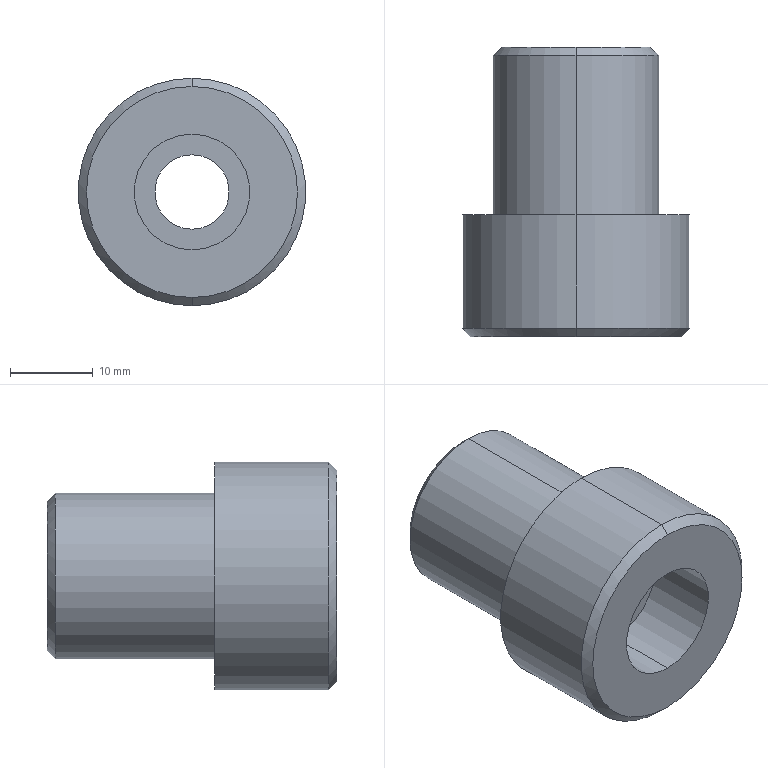Part | Creo | 1 solid | 16 faces | box 27.5 x 35 x 27.5 mm | volume 12011 mm3 | cylinder 8 | plane 4 | cone 4 | commonest cylinder face diameters 9 x2 14 x2 20 x2 27.5 x2
STEP:
#1=CARTESIAN_POINT('',(0.,0.,0.));
#2=DIRECTION('',(0.,0.,1.));
#3=DIRECTION('',(1.,0.,0.));
#4=AXIS2_PLACEMENT_3D('',#1,#2,#3);
#5=CARTESIAN_POINT('',(-64.528,-214.,-110.));
#6=VERTEX_POINT('',#5);
#7=CARTESIAN_POINT('',(-64.528,-214.,-92.));
#8=VERTEX_POINT('',#7);
#9=CARTESIAN_POINT('',(-64.528,-214.,-101.));
#10=DIRECTION('',(0.,1.,0.));
#11=DIRECTION('',(0.,0.,-1.));
#12=AXIS2_PLACEMENT_3D('',#9,#10,#11);
#13=CIRCLE('',#12,9.);
#14=EDGE_CURVE('',#6,#8,#13,.T.);
#15=ORIENTED_EDGE('',*,*,#14,.F.);
#16=CARTESIAN_POINT('',(-64.528,-214.,-101.));
#17=DIRECTION('',(0.,1.,0.));
#18=DIRECTION('',(0.,0.,1.));
#19=AXIS2_PLACEMENT_3D('',#16,#17,#18);
#20=CIRCLE('',#19,9.);
#21=EDGE_CURVE('',#8,#6,#20,.T.);
#22=ORIENTED_EDGE('',*,*,#21,.F.);
#23=EDGE_LOOP('',(#15,#22));
#24=FACE_OUTER_BOUND('',#23,.F.);
#25=CARTESIAN_POINT('',(-64.528,-214.,-96.5));
#26=VERTEX_POINT('',#25);
#27=CARTESIAN_POINT('',(-64.528,-214.,-105.5));
#28=VERTEX_POINT('',#27);
#29=CARTESIAN_POINT('',(-64.528,-214.,-101.));
#30=DIRECTION('',(0.,-1.,0.));
#31=DIRECTION('',(0.,0.,1.));
#32=AXIS2_PLACEMENT_3D('',#29,#30,#31);
#33=CIRCLE('',#32,4.5);
#34=EDGE_CURVE('',#26,#28,#33,.T.);
#35=ORIENTED_EDGE('',*,*,#34,.F.);
#36=CARTESIAN_POINT('',(-64.528,-214.,-101.));
#37=DIRECTION('',(0.,-1.,0.));
#38=DIRECTION('',(0.,0.,-1.));
#39=AXIS2_PLACEMENT_3D('',#36,#37,#38);
#40=CIRCLE('',#39,4.5);
#41=EDGE_CURVE('',#28,#26,#40,.T.);
#42=ORIENTED_EDGE('',*,*,#41,.F.);
#43=EDGE_LOOP('',(#35,#42));
#44=FACE_BOUND('',#43,.F.);
#45=CARTESIAN_POINT('',(-64.528,-214.,-101.));
#46=DIRECTION('',(0.,-1.,0.));
#47=DIRECTION('',(0.,0.,1.));
#48=AXIS2_PLACEMENT_3D('',#45,#46,#47);
#49=PLANE('',#48);
#50=ADVANCED_FACE('',(#24,#44),#49,.F.);
#51=CARTESIAN_POINT('',(-64.528,-215.,-111.));
#52=VERTEX_POINT('',#51);
#53=CARTESIAN_POINT('',(-64.528,-215.,-91.));
#54=VERTEX_POINT('',#53);
#55=CARTESIAN_POINT('',(-64.528,-215.,-101.));
#56=DIRECTION('',(0.,1.,0.));
#57=DIRECTION('',(0.,0.,-1.));
#58=AXIS2_PLACEMENT_3D('',#55,#56,#57);
#59=CIRCLE('',#58,10.);
#60=EDGE_CURVE('',#52,#54,#59,.T.);
#61=ORIENTED_EDGE('',*,*,#60,.F.);
#62=CARTESIAN_POINT('',(-64.528,-214.,-110.));
#63=DIRECTION('',(0.,-0.7071,-0.7071));
#64=VECTOR('',#63,1.414);
#65=LINE('',#62,#64);
#66=EDGE_CURVE('',#6,#52,#65,.T.);
#67=ORIENTED_EDGE('',*,*,#66,.F.);
#68=ORIENTED_EDGE('',*,*,#14,.T.);
#69=CARTESIAN_POINT('',(-64.528,-214.,-92.));
#70=DIRECTION('',(0.,-0.7071,0.7071));
#71=VECTOR('',#70,1.414);
#72=LINE('',#69,#71);
#73=EDGE_CURVE('',#8,#54,#72,.T.);
#74=ORIENTED_EDGE('',*,*,#73,.T.);
#75=EDGE_LOOP('',(#61,#67,#68,#74));
#76=FACE_OUTER_BOUND('',#75,.F.);
#77=CARTESIAN_POINT('',(-64.528,-214.5,-101.));
#78=DIRECTION('',(0.,-1.,0.));
#79=DIRECTION('',(0.,0.,-1.));
#80=AXIS2_PLACEMENT_3D('',#77,#78,#79);
#81=CONICAL_SURFACE('',#80,9.5,45.);
#82=ADVANCED_FACE('',(#76),#81,.T.);
#83=ORIENTED_EDGE('',*,*,#60,.T.);
#84=CARTESIAN_POINT('',(-64.528,-234.25,-91.));
#85=VERTEX_POINT('',#84);
#86=CARTESIAN_POINT('',(-64.528,-234.25,-91.));
#87=DIRECTION('',(0.,1.,0.));
#88=VECTOR('',#87,19.25);
#89=LINE('',#86,#88);
#90=EDGE_CURVE('',#85,#54,#89,.T.);
#91=ORIENTED_EDGE('',*,*,#90,.F.);
#92=CARTESIAN_POINT('',(-64.528,-234.25,-111.));
#93=VERTEX_POINT('',#92);
#94=CARTESIAN_POINT('',(-64.528,-234.25,-101.));
#95=DIRECTION('',(0.,-1.,0.));
#96=DIRECTION('',(0.,0.,1.));
#97=AXIS2_PLACEMENT_3D('',#94,#95,#96);
#98=CIRCLE('',#97,10.);
#99=EDGE_CURVE('',#85,#93,#98,.T.);
#100=ORIENTED_EDGE('',*,*,#99,.T.);
#101=CARTESIAN_POINT('',(-64.528,-234.25,-111.));
#102=DIRECTION('',(0.,1.,0.));
#103=VECTOR('',#102,19.25);
#104=LINE('',#101,#103);
#105=EDGE_CURVE('',#93,#52,#104,.T.);
#106=ORIENTED_EDGE('',*,*,#105,.T.);
#107=EDGE_LOOP('',(#83,#91,#100,#106));
#108=FACE_OUTER_BOUND('',#107,.F.);
#109=CARTESIAN_POINT('',(-64.528,-249.,-101.));
#110=DIRECTION('',(0.,1.,0.));
#111=DIRECTION('',(0.,0.,-1.));
#112=AXIS2_PLACEMENT_3D('',#109,#110,#111);
#113=CYLINDRICAL_SURFACE('',#112,10.);
#114=ADVANCED_FACE('',(#108),#113,.T.);
#115=CARTESIAN_POINT('',(-64.528,-215.,-101.));
#116=DIRECTION('',(0.,1.,0.));
#117=DIRECTION('',(0.,0.,1.));
#118=AXIS2_PLACEMENT_3D('',#115,#116,#117);
#119=CIRCLE('',#118,10.);
#120=EDGE_CURVE('',#54,#52,#119,.T.);
#121=ORIENTED_EDGE('',*,*,#120,.T.);
#122=ORIENTED_EDGE('',*,*,#105,.F.);
#123=CARTESIAN_POINT('',(-64.528,-234.25,-101.));
#124=DIRECTION('',(0.,-1.,0.));
#125=DIRECTION('',(0.,0.,-1.));
#126=AXIS2_PLACEMENT_3D('',#123,#124,#125);
#127=CIRCLE('',#126,10.);
#128=EDGE_CURVE('',#93,#85,#127,.T.);
#129=ORIENTED_EDGE('',*,*,#128,.T.);
#130=ORIENTED_EDGE('',*,*,#90,.T.);
#131=EDGE_LOOP('',(#121,#122,#129,#130));
#132=FACE_OUTER_BOUND('',#131,.F.);
#133=CARTESIAN_POINT('',(-64.528,-249.,-101.));
#134=DIRECTION('',(0.,1.,0.));
#135=DIRECTION('',(0.,0.,-1.));
#136=AXIS2_PLACEMENT_3D('',#133,#134,#135);
#137=CYLINDRICAL_SURFACE('',#136,10.);
#138=ADVANCED_FACE('',(#132),#137,.T.);
#139=ORIENTED_EDGE('',*,*,#120,.F.);
#140=ORIENTED_EDGE('',*,*,#73,.F.);
#141=ORIENTED_EDGE('',*,*,#21,.T.);
#142=ORIENTED_EDGE('',*,*,#66,.T.);
#143=EDGE_LOOP('',(#139,#140,#141,#142));
#144=FACE_OUTER_BOUND('',#143,.F.);
#145=CARTESIAN_POINT('',(-64.528,-214.5,-101.));
#146=DIRECTION('',(0.,-1.,0.));
#147=DIRECTION('',(0.,0.,-1.));
#148=AXIS2_PLACEMENT_3D('',#145,#146,#147);
#149=CONICAL_SURFACE('',#148,9.5,45.);
#150=ADVANCED_FACE('',(#144),#149,.T.);
#151=CARTESIAN_POINT('',(-64.528,-234.25,-114.75));
#152=VERTEX_POINT('',#151);
#153=CARTESIAN_POINT('',(-64.528,-234.25,-87.25));
#154=VERTEX_POINT('',#153);
#155=CARTESIAN_POINT('',(-64.528,-234.25,-101.));
#156=DIRECTION('',(0.,1.,0.));
#157=DIRECTION('',(0.,0.,-1.));
#158=AXIS2_PLACEMENT_3D('',#155,#156,#157);
#159=CIRCLE('',#158,13.75);
#160=EDGE_CURVE('',#152,#154,#159,.T.);
#161=ORIENTED_EDGE('',*,*,#160,.F.);
#162=CARTESIAN_POINT('',(-64.528,-234.25,-101.));
#163=DIRECTION('',(0.,1.,0.));
#164=DIRECTION('',(0.,0.,1.));
#165=AXIS2_PLACEMENT_3D('',#162,#163,#164);
#166=CIRCLE('',#165,13.75);
#167=EDGE_CURVE('',#154,#152,#166,.T.);
#168=ORIENTED_EDGE('',*,*,#167,.F.);
#169=EDGE_LOOP('',(#161,#168));
#170=FACE_OUTER_BOUND('',#169,.F.);
#171=ORIENTED_EDGE('',*,*,#99,.F.);
#172=ORIENTED_EDGE('',*,*,#128,.F.);
#173=EDGE_LOOP('',(#171,#172));
#174=FACE_BOUND('',#173,.F.);
#175=CARTESIAN_POINT('',(-64.528,-234.25,-101.));
#176=DIRECTION('',(0.,-1.,0.));
#177=DIRECTION('',(0.,0.,1.));
#178=AXIS2_PLACEMENT_3D('',#175,#176,#177);
#179=PLANE('',#178);
#180=ADVANCED_FACE('',(#170,#174),#179,.F.);
#181=CARTESIAN_POINT('',(-64.528,-248.,-87.25));
#182=VERTEX_POINT('',#181);
#183=CARTESIAN_POINT('',(-64.528,-248.,-114.75));
#184=VERTEX_POINT('',#183);
#185=CARTESIAN_POINT('',(-64.528,-248.,-101.));
#186=DIRECTION('',(0.,-1.,0.));
#187=DIRECTION('',(0.,0.,1.));
#188=AXIS2_PLACEMENT_3D('',#185,#186,#187);
#189=CIRCLE('',#188,13.75);
#190=EDGE_CURVE('',#182,#184,#189,.T.);
#191=ORIENTED_EDGE('',*,*,#190,.T.);
#192=CARTESIAN_POINT('',(-64.528,-248.,-114.75));
#193=DIRECTION('',(0.,1.,0.));
#194=VECTOR('',#193,13.75);
#195=LINE('',#192,#194);
#196=EDGE_CURVE('',#184,#152,#195,.T.);
#197=ORIENTED_EDGE('',*,*,#196,.T.);
#198=ORIENTED_EDGE('',*,*,#160,.T.);
#199=CARTESIAN_POINT('',(-64.528,-248.,-87.25));
#200=DIRECTION('',(0.,1.,0.));
#201=VECTOR('',#200,13.75);
#202=LINE('',#199,#201);
#203=EDGE_CURVE('',#182,#154,#202,.T.);
#204=ORIENTED_EDGE('',*,*,#203,.F.);
#205=EDGE_LOOP('',(#191,#197,#198,#204));
#206=FACE_OUTER_BOUND('',#205,.F.);
#207=CARTESIAN_POINT('',(-64.528,-249.,-101.));
#208=DIRECTION('',(0.,1.,0.));
#209=DIRECTION('',(0.,0.,-1.));
#210=AXIS2_PLACEMENT_3D('',#207,#208,#209);
#211=CYLINDRICAL_SURFACE('',#210,13.75);
#212=ADVANCED_FACE('',(#206),#211,.T.);
#213=ORIENTED_EDGE('',*,*,#190,.F.);
#214=CARTESIAN_POINT('',(-64.528,-249.,-88.25));
#215=VERTEX_POINT('',#214);
#216=CARTESIAN_POINT('',(-64.528,-249.,-88.25));
#217=DIRECTION('',(0.,0.7071,0.7071));
#218=VECTOR('',#217,1.414);
#219=LINE('',#216,#218);
#220=EDGE_CURVE('',#215,#182,#219,.T.);
#221=ORIENTED_EDGE('',*,*,#220,.F.);
#222=CARTESIAN_POINT('',(-64.528,-249.,-113.75));
#223=VERTEX_POINT('',#222);
#224=CARTESIAN_POINT('',(-64.528,-249.,-101.));
#225=DIRECTION('',(0.,-1.,0.));
#226=DIRECTION('',(0.,0.,1.));
#227=AXIS2_PLACEMENT_3D('',#224,#225,#226);
#228=CIRCLE('',#227,12.75);
#229=EDGE_CURVE('',#215,#223,#228,.T.);
#230=ORIENTED_EDGE('',*,*,#229,.T.);
#231=CARTESIAN_POINT('',(-64.528,-249.,-113.75));
#232=DIRECTION('',(0.,0.7071,-0.7071));
#233=VECTOR('',#232,1.414);
#234=LINE('',#231,#233);
#235=EDGE_CURVE('',#223,#184,#234,.T.);
#236=ORIENTED_EDGE('',*,*,#235,.T.);
#237=EDGE_LOOP('',(#213,#221,#230,#236));
#238=FACE_OUTER_BOUND('',#237,.F.);
#239=CARTESIAN_POINT('',(-64.528,-248.5,-101.));
#240=DIRECTION('',(0.,1.,0.));
#241=DIRECTION('',(0.,0.,1.));
#242=AXIS2_PLACEMENT_3D('',#239,#240,#241);
#243=CONICAL_SURFACE('',#242,13.25,45.);
#244=ADVANCED_FACE('',(#238),#243,.T.);
#245=CARTESIAN_POINT('',(-64.528,-248.,-101.));
#246=DIRECTION('',(0.,-1.,0.));
#247=DIRECTION('',(0.,0.,-1.));
#248=AXIS2_PLACEMENT_3D('',#245,#246,#247);
#249=CIRCLE('',#248,13.75);
#250=EDGE_CURVE('',#184,#182,#249,.T.);
#251=ORIENTED_EDGE('',*,*,#250,.F.);
#252=ORIENTED_EDGE('',*,*,#235,.F.);
#253=CARTESIAN_POINT('',(-64.528,-249.,-101.));
#254=DIRECTION('',(0.,-1.,0.));
#255=DIRECTION('',(0.,0.,-1.));
#256=AXIS2_PLACEMENT_3D('',#253,#254,#255);
#257=CIRCLE('',#256,12.75);
#258=EDGE_CURVE('',#223,#215,#257,.T.);
#259=ORIENTED_EDGE('',*,*,#258,.T.);
#260=ORIENTED_EDGE('',*,*,#220,.T.);
#261=EDGE_LOOP('',(#251,#252,#259,#260));
#262=FACE_OUTER_BOUND('',#261,.F.);
#263=CARTESIAN_POINT('',(-64.528,-248.5,-101.));
#264=DIRECTION('',(0.,1.,0.));
#265=DIRECTION('',(0.,0.,1.));
#266=AXIS2_PLACEMENT_3D('',#263,#264,#265);
#267=CONICAL_SURFACE('',#266,13.25,45.);
#268=ADVANCED_FACE('',(#262),#267,.T.);
#269=ORIENTED_EDGE('',*,*,#250,.T.);
#270=ORIENTED_EDGE('',*,*,#203,.T.);
#271=ORIENTED_EDGE('',*,*,#167,.T.);
#272=ORIENTED_EDGE('',*,*,#196,.F.);
#273=EDGE_LOOP('',(#269,#270,#271,#272));
#274=FACE_OUTER_BOUND('',#273,.F.);
#275=CARTESIAN_POINT('',(-64.528,-249.,-101.));
#276=DIRECTION('',(0.,1.,0.));
#277=DIRECTION('',(0.,0.,-1.));
#278=AXIS2_PLACEMENT_3D('',#275,#276,#277);
#279=CYLINDRICAL_SURFACE('',#278,13.75);
#280=ADVANCED_FACE('',(#274),#279,.T.);
#281=ORIENTED_EDGE('',*,*,#258,.F.);
#282=ORIENTED_EDGE('',*,*,#229,.F.);
#283=EDGE_LOOP('',(#281,#282));
#284=FACE_OUTER_BOUND('',#283,.F.);
#285=CARTESIAN_POINT('',(-64.528,-249.,-108.));
#286=VERTEX_POINT('',#285);
#287=CARTESIAN_POINT('',(-64.528,-249.,-94.));
#288=VERTEX_POINT('',#287);
#289=CARTESIAN_POINT('',(-64.528,-249.,-101.));
#290=DIRECTION('',(0.,1.,0.));
#291=DIRECTION('',(0.,0.,-1.));
#292=AXIS2_PLACEMENT_3D('',#289,#290,#291);
#293=CIRCLE('',#292,7.);
#294=EDGE_CURVE('',#286,#288,#293,.T.);
#295=ORIENTED_EDGE('',*,*,#294,.F.);
#296=CARTESIAN_POINT('',(-64.528,-249.,-101.));
#297=DIRECTION('',(0.,1.,0.));
#298=DIRECTION('',(0.,0.,1.));
#299=AXIS2_PLACEMENT_3D('',#296,#297,#298);
#300=CIRCLE('',#299,7.);
#301=EDGE_CURVE('',#288,#286,#300,.T.);
#302=ORIENTED_EDGE('',*,*,#301,.F.);
#303=EDGE_LOOP('',(#295,#302));
#304=FACE_BOUND('',#303,.F.);
#305=CARTESIAN_POINT('',(-64.528,-249.,-101.));
#306=DIRECTION('',(0.,-1.,0.));
#307=DIRECTION('',(0.,0.,1.));
#308=AXIS2_PLACEMENT_3D('',#305,#306,#307);
#309=PLANE('',#308);
#310=ADVANCED_FACE('',(#284,#304),#309,.T.);
#311=CARTESIAN_POINT('',(-64.528,-240.,-94.));
#312=VERTEX_POINT('',#311);
#313=CARTESIAN_POINT('',(-64.528,-240.,-108.));
#314=VERTEX_POINT('',#313);
#315=CARTESIAN_POINT('',(-64.528,-240.,-101.));
#316=DIRECTION('',(0.,-1.,0.));
#317=DIRECTION('',(0.,0.,1.));
#318=AXIS2_PLACEMENT_3D('',#315,#316,#317);
#319=CIRCLE('',#318,7.);
#320=EDGE_CURVE('',#312,#314,#319,.T.);
#321=ORIENTED_EDGE('',*,*,#320,.T.);
#322=CARTESIAN_POINT('',(-64.528,-249.,-108.));
#323=DIRECTION('',(0.,1.,0.));
#324=VECTOR('',#323,9.);
#325=LINE('',#322,#324);
#326=EDGE_CURVE('',#286,#314,#325,.T.);
#327=ORIENTED_EDGE('',*,*,#326,.F.);
#328=ORIENTED_EDGE('',*,*,#294,.T.);
#329=CARTESIAN_POINT('',(-64.528,-249.,-94.));
#330=DIRECTION('',(0.,1.,0.));
#331=VECTOR('',#330,9.);
#332=LINE('',#329,#331);
#333=EDGE_CURVE('',#288,#312,#332,.T.);
#334=ORIENTED_EDGE('',*,*,#333,.T.);
#335=EDGE_LOOP('',(#321,#327,#328,#334));
#336=FACE_OUTER_BOUND('',#335,.F.);
#337=CARTESIAN_POINT('',(-64.528,-249.,-101.));
#338=DIRECTION('',(0.,1.,0.));
#339=DIRECTION('',(0.,0.,-1.));
#340=AXIS2_PLACEMENT_3D('',#337,#338,#339);
#341=CYLINDRICAL_SURFACE('',#340,7.);
#342=ADVANCED_FACE('',(#336),#341,.F.);
#343=CARTESIAN_POINT('',(-64.528,-240.,-101.));
#344=DIRECTION('',(0.,-1.,0.));
#345=DIRECTION('',(0.,0.,-1.));
#346=AXIS2_PLACEMENT_3D('',#343,#344,#345);
#347=CIRCLE('',#346,7.);
#348=EDGE_CURVE('',#314,#312,#347,.T.);
#349=ORIENTED_EDGE('',*,*,#348,.F.);
#350=ORIENTED_EDGE('',*,*,#320,.F.);
#351=EDGE_LOOP('',(#349,#350));
#352=FACE_OUTER_BOUND('',#351,.F.);
#353=CARTESIAN_POINT('',(-64.528,-240.,-105.5));
#354=VERTEX_POINT('',#353);
#355=CARTESIAN_POINT('',(-64.528,-240.,-96.5));
#356=VERTEX_POINT('',#355);
#357=CARTESIAN_POINT('',(-64.528,-240.,-101.));
#358=DIRECTION('',(0.,1.,0.));
#359=DIRECTION('',(0.,0.,-1.));
#360=AXIS2_PLACEMENT_3D('',#357,#358,#359);
#361=CIRCLE('',#360,4.5);
#362=EDGE_CURVE('',#354,#356,#361,.T.);
#363=ORIENTED_EDGE('',*,*,#362,.F.);
#364=CARTESIAN_POINT('',(-64.528,-240.,-101.));
#365=DIRECTION('',(0.,1.,0.));
#366=DIRECTION('',(0.,0.,1.));
#367=AXIS2_PLACEMENT_3D('',#364,#365,#366);
#368=CIRCLE('',#367,4.5);
#369=EDGE_CURVE('',#356,#354,#368,.T.);
#370=ORIENTED_EDGE('',*,*,#369,.F.);
#371=EDGE_LOOP('',(#363,#370));
#372=FACE_BOUND('',#371,.F.);
#373=CARTESIAN_POINT('',(-64.528,-240.,-101.));
#374=DIRECTION('',(0.,1.,0.));
#375=DIRECTION('',(0.,0.,-1.));
#376=AXIS2_PLACEMENT_3D('',#373,#374,#375);
#377=PLANE('',#376);
#378=ADVANCED_FACE('',(#352,#372),#377,.F.);
#379=ORIENTED_EDGE('',*,*,#362,.T.);
#380=CARTESIAN_POINT('',(-64.528,-240.,-96.5));
#381=DIRECTION('',(0.,1.,0.));
#382=VECTOR('',#381,26.);
#383=LINE('',#380,#382);
#384=EDGE_CURVE('',#356,#26,#383,.T.);
#385=ORIENTED_EDGE('',*,*,#384,.T.);
#386=ORIENTED_EDGE('',*,*,#34,.T.);
#387=CARTESIAN_POINT('',(-64.528,-240.,-105.5));
#388=DIRECTION('',(0.,1.,0.));
#389=VECTOR('',#388,26.);
#390=LINE('',#387,#389);
#391=EDGE_CURVE('',#354,#28,#390,.T.);
#392=ORIENTED_EDGE('',*,*,#391,.F.);
#393=EDGE_LOOP('',(#379,#385,#386,#392));
#394=FACE_OUTER_BOUND('',#393,.F.);
#395=CARTESIAN_POINT('',(-64.528,-49.,-101.));
#396=DIRECTION('',(0.,1.,0.));
#397=DIRECTION('',(0.,0.,-1.));
#398=AXIS2_PLACEMENT_3D('',#395,#396,#397);
#399=CYLINDRICAL_SURFACE('',#398,4.5);
#400=ADVANCED_FACE('',(#394),#399,.F.);
#401=ORIENTED_EDGE('',*,*,#369,.T.);
#402=ORIENTED_EDGE('',*,*,#391,.T.);
#403=ORIENTED_EDGE('',*,*,#41,.T.);
#404=ORIENTED_EDGE('',*,*,#384,.F.);
#405=EDGE_LOOP('',(#401,#402,#403,#404));
#406=FACE_OUTER_BOUND('',#405,.F.);
#407=CARTESIAN_POINT('',(-64.528,-49.,-101.));
#408=DIRECTION('',(0.,1.,0.));
#409=DIRECTION('',(0.,0.,-1.));
#410=AXIS2_PLACEMENT_3D('',#407,#408,#409);
#411=CYLINDRICAL_SURFACE('',#410,4.5);
#412=ADVANCED_FACE('',(#406),#411,.F.);
#413=ORIENTED_EDGE('',*,*,#348,.T.);
#414=ORIENTED_EDGE('',*,*,#333,.F.);
#415=ORIENTED_EDGE('',*,*,#301,.T.);
#416=ORIENTED_EDGE('',*,*,#326,.T.);
#417=EDGE_LOOP('',(#413,#414,#415,#416));
#418=FACE_OUTER_BOUND('',#417,.F.);
#419=CARTESIAN_POINT('',(-64.528,-249.,-101.));
#420=DIRECTION('',(0.,1.,0.));
#421=DIRECTION('',(0.,0.,-1.));
#422=AXIS2_PLACEMENT_3D('',#419,#420,#421);
#423=CYLINDRICAL_SURFACE('',#422,7.);
#424=ADVANCED_FACE('',(#418),#423,.F.);
#425=CLOSED_SHELL('',(#50,#82,#114,#138,#150,#180,#212,#244,#268,#280,#310,#342,#378,#400,#412,#424));
#426=MANIFOLD_SOLID_BREP('',#425);
#427=(LENGTH_UNIT()NAMED_UNIT(*)SI_UNIT(.MILLI.,.METRE.));
#428=UNCERTAINTY_MEASURE_WITH_UNIT(LENGTH_MEASURE(0.005232),#427,'','');
#429=(NAMED_UNIT(*)PLANE_ANGLE_UNIT()SI_UNIT($,.RADIAN.));
#430=PLANE_ANGLE_MEASURE_WITH_UNIT(PLANE_ANGLE_MEASURE(0.01745),#429);
#431=(CONVERSION_BASED_UNIT('DEGREE',#430)NAMED_UNIT(*)PLANE_ANGLE_UNIT());
#432=(NAMED_UNIT(*)SI_UNIT($,.STERADIAN.)SOLID_ANGLE_UNIT());
#433=(GEOMETRIC_REPRESENTATION_CONTEXT(3)GLOBAL_UNCERTAINTY_ASSIGNED_CONTEXT((#428))GLOBAL_UNIT_ASSIGNED_CONTEXT((#427,#431,#432))REPRESENTATION_CONTEXT('',''));
#434=ADVANCED_BREP_SHAPE_REPRESENTATION('',(#4,#426),#433);